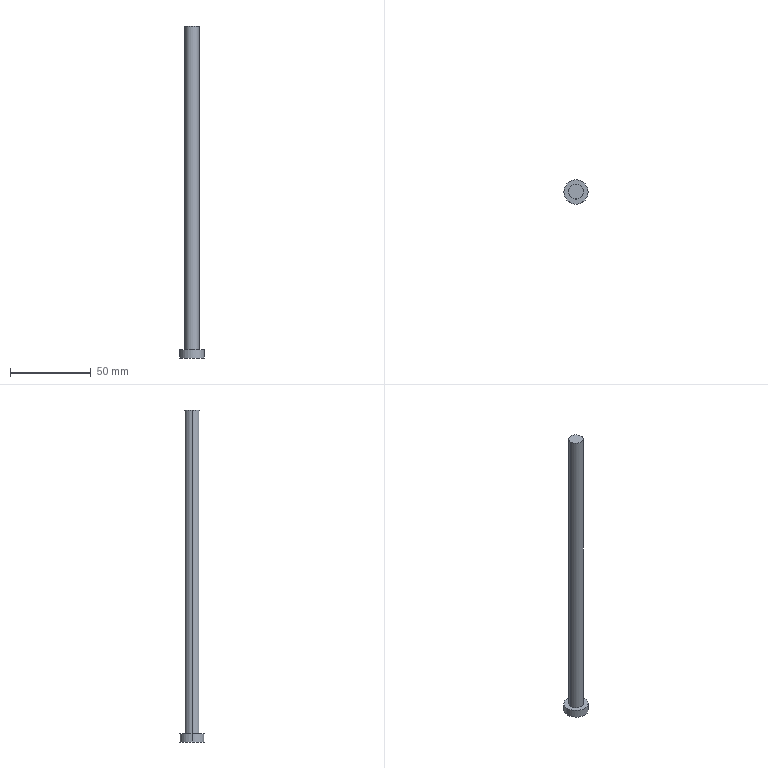Part | Creo | 1 solid | 7 faces | box 15 x 15 x 205 mm | volume 13607 mm3 | cylinder 4 | plane 3 | commonest cylinder face diameters 9 x2 15 x2
STEP:
#1=CARTESIAN_POINT('',(-4.5,0.,-220.5));
#2=VERTEX_POINT('',#1);
#3=CARTESIAN_POINT('',(4.5,0.,-220.5));
#4=VERTEX_POINT('',#3);
#5=CARTESIAN_POINT('',(0.,0.,-220.5));
#6=DIRECTION('',(0.,0.,-1.));
#7=DIRECTION('',(-1.,0.,0.));
#8=AXIS2_PLACEMENT_3D('',#5,#6,#7);
#9=CIRCLE('',#8,4.5);
#10=EDGE_CURVE('',#2,#4,#9,.T.);
#11=ORIENTED_EDGE('',*,*,#10,.T.);
#12=CARTESIAN_POINT('',(4.5,0.,-20.5));
#13=VERTEX_POINT('',#12);
#14=CARTESIAN_POINT('',(4.5,0.,-220.5));
#15=DIRECTION('',(0.,0.,1.));
#16=VECTOR('',#15,200.);
#17=LINE('',#14,#16);
#18=EDGE_CURVE('',#4,#13,#17,.T.);
#19=ORIENTED_EDGE('',*,*,#18,.T.);
#20=CARTESIAN_POINT('',(-4.5,0.,-20.5));
#21=VERTEX_POINT('',#20);
#22=CARTESIAN_POINT('',(0.,0.,-20.5));
#23=DIRECTION('',(0.,0.,1.));
#24=DIRECTION('',(1.,0.,0.));
#25=AXIS2_PLACEMENT_3D('',#22,#23,#24);
#26=CIRCLE('',#25,4.5);
#27=EDGE_CURVE('',#13,#21,#26,.T.);
#28=ORIENTED_EDGE('',*,*,#27,.T.);
#29=CARTESIAN_POINT('',(-4.5,0.,-220.5));
#30=DIRECTION('',(0.,0.,1.));
#31=VECTOR('',#30,200.);
#32=LINE('',#29,#31);
#33=EDGE_CURVE('',#2,#21,#32,.T.);
#34=ORIENTED_EDGE('',*,*,#33,.F.);
#35=EDGE_LOOP('',(#11,#19,#28,#34));
#36=FACE_OUTER_BOUND('',#35,.F.);
#37=CARTESIAN_POINT('',(0.,0.,-250.296));
#38=DIRECTION('',(0.,0.,1.));
#39=DIRECTION('',(1.,0.,0.));
#40=AXIS2_PLACEMENT_3D('',#37,#38,#39);
#41=CYLINDRICAL_SURFACE('',#40,4.5);
#42=ADVANCED_FACE('',(#36),#41,.T.);
#43=CARTESIAN_POINT('',(7.5,0.,-220.5));
#44=VERTEX_POINT('',#43);
#45=CARTESIAN_POINT('',(-7.5,0.,-220.5));
#46=VERTEX_POINT('',#45);
#47=CARTESIAN_POINT('',(0.,0.,-220.5));
#48=DIRECTION('',(0.,0.,1.));
#49=DIRECTION('',(1.,0.,0.));
#50=AXIS2_PLACEMENT_3D('',#47,#48,#49);
#51=CIRCLE('',#50,7.5);
#52=EDGE_CURVE('',#44,#46,#51,.T.);
#53=ORIENTED_EDGE('',*,*,#52,.F.);
#54=CARTESIAN_POINT('',(0.,0.,-220.5));
#55=DIRECTION('',(0.,0.,1.));
#56=DIRECTION('',(-1.,0.,0.));
#57=AXIS2_PLACEMENT_3D('',#54,#55,#56);
#58=CIRCLE('',#57,7.5);
#59=EDGE_CURVE('',#46,#44,#58,.T.);
#60=ORIENTED_EDGE('',*,*,#59,.F.);
#61=EDGE_LOOP('',(#53,#60));
#62=FACE_OUTER_BOUND('',#61,.F.);
#63=CARTESIAN_POINT('',(0.,0.,-220.5));
#64=DIRECTION('',(0.,0.,-1.));
#65=DIRECTION('',(1.,0.,0.));
#66=AXIS2_PLACEMENT_3D('',#63,#64,#65);
#67=CIRCLE('',#66,4.5);
#68=EDGE_CURVE('',#4,#2,#67,.T.);
#69=ORIENTED_EDGE('',*,*,#68,.F.);
#70=ORIENTED_EDGE('',*,*,#10,.F.);
#71=EDGE_LOOP('',(#69,#70));
#72=FACE_BOUND('',#71,.F.);
#73=CARTESIAN_POINT('',(0.,0.,-220.5));
#74=DIRECTION('',(0.,0.,1.));
#75=DIRECTION('',(1.,0.,0.));
#76=AXIS2_PLACEMENT_3D('',#73,#74,#75);
#77=PLANE('',#76);
#78=ADVANCED_FACE('',(#62,#72),#77,.T.);
#79=CARTESIAN_POINT('',(-7.5,0.,-225.5));
#80=VERTEX_POINT('',#79);
#81=CARTESIAN_POINT('',(7.5,0.,-225.5));
#82=VERTEX_POINT('',#81);
#83=CARTESIAN_POINT('',(0.,0.,-225.5));
#84=DIRECTION('',(0.,0.,-1.));
#85=DIRECTION('',(-1.,0.,0.));
#86=AXIS2_PLACEMENT_3D('',#83,#84,#85);
#87=CIRCLE('',#86,7.5);
#88=EDGE_CURVE('',#80,#82,#87,.T.);
#89=ORIENTED_EDGE('',*,*,#88,.T.);
#90=CARTESIAN_POINT('',(7.5,0.,-225.5));
#91=DIRECTION('',(0.,0.,1.));
#92=VECTOR('',#91,5.);
#93=LINE('',#90,#92);
#94=EDGE_CURVE('',#82,#44,#93,.T.);
#95=ORIENTED_EDGE('',*,*,#94,.T.);
#96=ORIENTED_EDGE('',*,*,#52,.T.);
#97=CARTESIAN_POINT('',(-7.5,0.,-225.5));
#98=DIRECTION('',(0.,0.,1.));
#99=VECTOR('',#98,5.);
#100=LINE('',#97,#99);
#101=EDGE_CURVE('',#80,#46,#100,.T.);
#102=ORIENTED_EDGE('',*,*,#101,.F.);
#103=EDGE_LOOP('',(#89,#95,#96,#102));
#104=FACE_OUTER_BOUND('',#103,.F.);
#105=CARTESIAN_POINT('',(0.,0.,-231.77));
#106=DIRECTION('',(0.,0.,1.));
#107=DIRECTION('',(1.,0.,0.));
#108=AXIS2_PLACEMENT_3D('',#105,#106,#107);
#109=CYLINDRICAL_SURFACE('',#108,7.5);
#110=ADVANCED_FACE('',(#104),#109,.T.);
#111=CARTESIAN_POINT('',(0.,0.,-225.5));
#112=DIRECTION('',(0.,0.,-1.));
#113=DIRECTION('',(1.,0.,0.));
#114=AXIS2_PLACEMENT_3D('',#111,#112,#113);
#115=CIRCLE('',#114,7.5);
#116=EDGE_CURVE('',#82,#80,#115,.T.);
#117=ORIENTED_EDGE('',*,*,#116,.F.);
#118=ORIENTED_EDGE('',*,*,#88,.F.);
#119=EDGE_LOOP('',(#117,#118));
#120=FACE_OUTER_BOUND('',#119,.F.);
#121=CARTESIAN_POINT('',(0.,0.,-225.5));
#122=DIRECTION('',(0.,0.,1.));
#123=DIRECTION('',(1.,0.,0.));
#124=AXIS2_PLACEMENT_3D('',#121,#122,#123);
#125=PLANE('',#124);
#126=ADVANCED_FACE('',(#120),#125,.F.);
#127=ORIENTED_EDGE('',*,*,#116,.T.);
#128=ORIENTED_EDGE('',*,*,#101,.T.);
#129=ORIENTED_EDGE('',*,*,#59,.T.);
#130=ORIENTED_EDGE('',*,*,#94,.F.);
#131=EDGE_LOOP('',(#127,#128,#129,#130));
#132=FACE_OUTER_BOUND('',#131,.F.);
#133=CARTESIAN_POINT('',(0.,0.,-231.77));
#134=DIRECTION('',(0.,0.,1.));
#135=DIRECTION('',(1.,0.,0.));
#136=AXIS2_PLACEMENT_3D('',#133,#134,#135);
#137=CYLINDRICAL_SURFACE('',#136,7.5);
#138=ADVANCED_FACE('',(#132),#137,.T.);
#139=ORIENTED_EDGE('',*,*,#68,.T.);
#140=ORIENTED_EDGE('',*,*,#33,.T.);
#141=CARTESIAN_POINT('',(0.,0.,-20.5));
#142=DIRECTION('',(0.,0.,1.));
#143=DIRECTION('',(-1.,0.,0.));
#144=AXIS2_PLACEMENT_3D('',#141,#142,#143);
#145=CIRCLE('',#144,4.5);
#146=EDGE_CURVE('',#21,#13,#145,.T.);
#147=ORIENTED_EDGE('',*,*,#146,.T.);
#148=ORIENTED_EDGE('',*,*,#18,.F.);
#149=EDGE_LOOP('',(#139,#140,#147,#148));
#150=FACE_OUTER_BOUND('',#149,.F.);
#151=CARTESIAN_POINT('',(0.,0.,-250.296));
#152=DIRECTION('',(0.,0.,1.));
#153=DIRECTION('',(1.,0.,0.));
#154=AXIS2_PLACEMENT_3D('',#151,#152,#153);
#155=CYLINDRICAL_SURFACE('',#154,4.5);
#156=ADVANCED_FACE('',(#150),#155,.T.);
#157=ORIENTED_EDGE('',*,*,#27,.F.);
#158=ORIENTED_EDGE('',*,*,#146,.F.);
#159=EDGE_LOOP('',(#157,#158));
#160=FACE_OUTER_BOUND('',#159,.F.);
#161=CARTESIAN_POINT('',(4.5,0.,-20.5));
#162=DIRECTION('',(0.,0.,-1.));
#163=DIRECTION('',(-1.,0.,0.));
#164=AXIS2_PLACEMENT_3D('',#161,#162,#163);
#165=PLANE('',#164);
#166=ADVANCED_FACE('',(#160),#165,.F.);
#167=CLOSED_SHELL('',(#42,#78,#110,#126,#138,#156,#166));
#168=MANIFOLD_SOLID_BREP('',#167);
#169=(LENGTH_UNIT()NAMED_UNIT(*)SI_UNIT(.MILLI.,.METRE.));
#170=UNCERTAINTY_MEASURE_WITH_UNIT(LENGTH_MEASURE(0.02061),#169,'','');
#171=(NAMED_UNIT(*)PLANE_ANGLE_UNIT()SI_UNIT($,.RADIAN.));
#172=PLANE_ANGLE_MEASURE_WITH_UNIT(PLANE_ANGLE_MEASURE(0.01745),#171);
#173=(CONVERSION_BASED_UNIT('DEGREE',#172)NAMED_UNIT(*)PLANE_ANGLE_UNIT());
#174=(NAMED_UNIT(*)SI_UNIT($,.STERADIAN.)SOLID_ANGLE_UNIT());
#175=(GEOMETRIC_REPRESENTATION_CONTEXT(3)GLOBAL_UNCERTAINTY_ASSIGNED_CONTEXT((#170))GLOBAL_UNIT_ASSIGNED_CONTEXT((#169,#173,#174))REPRESENTATION_CONTEXT('',''));
#176=ADVANCED_BREP_SHAPE_REPRESENTATION('',(#168),#175);